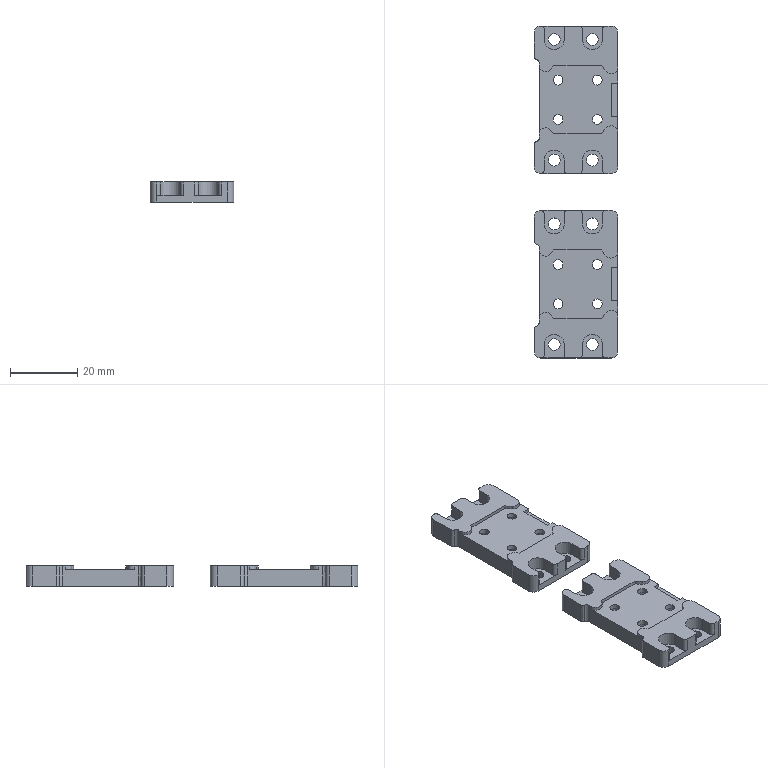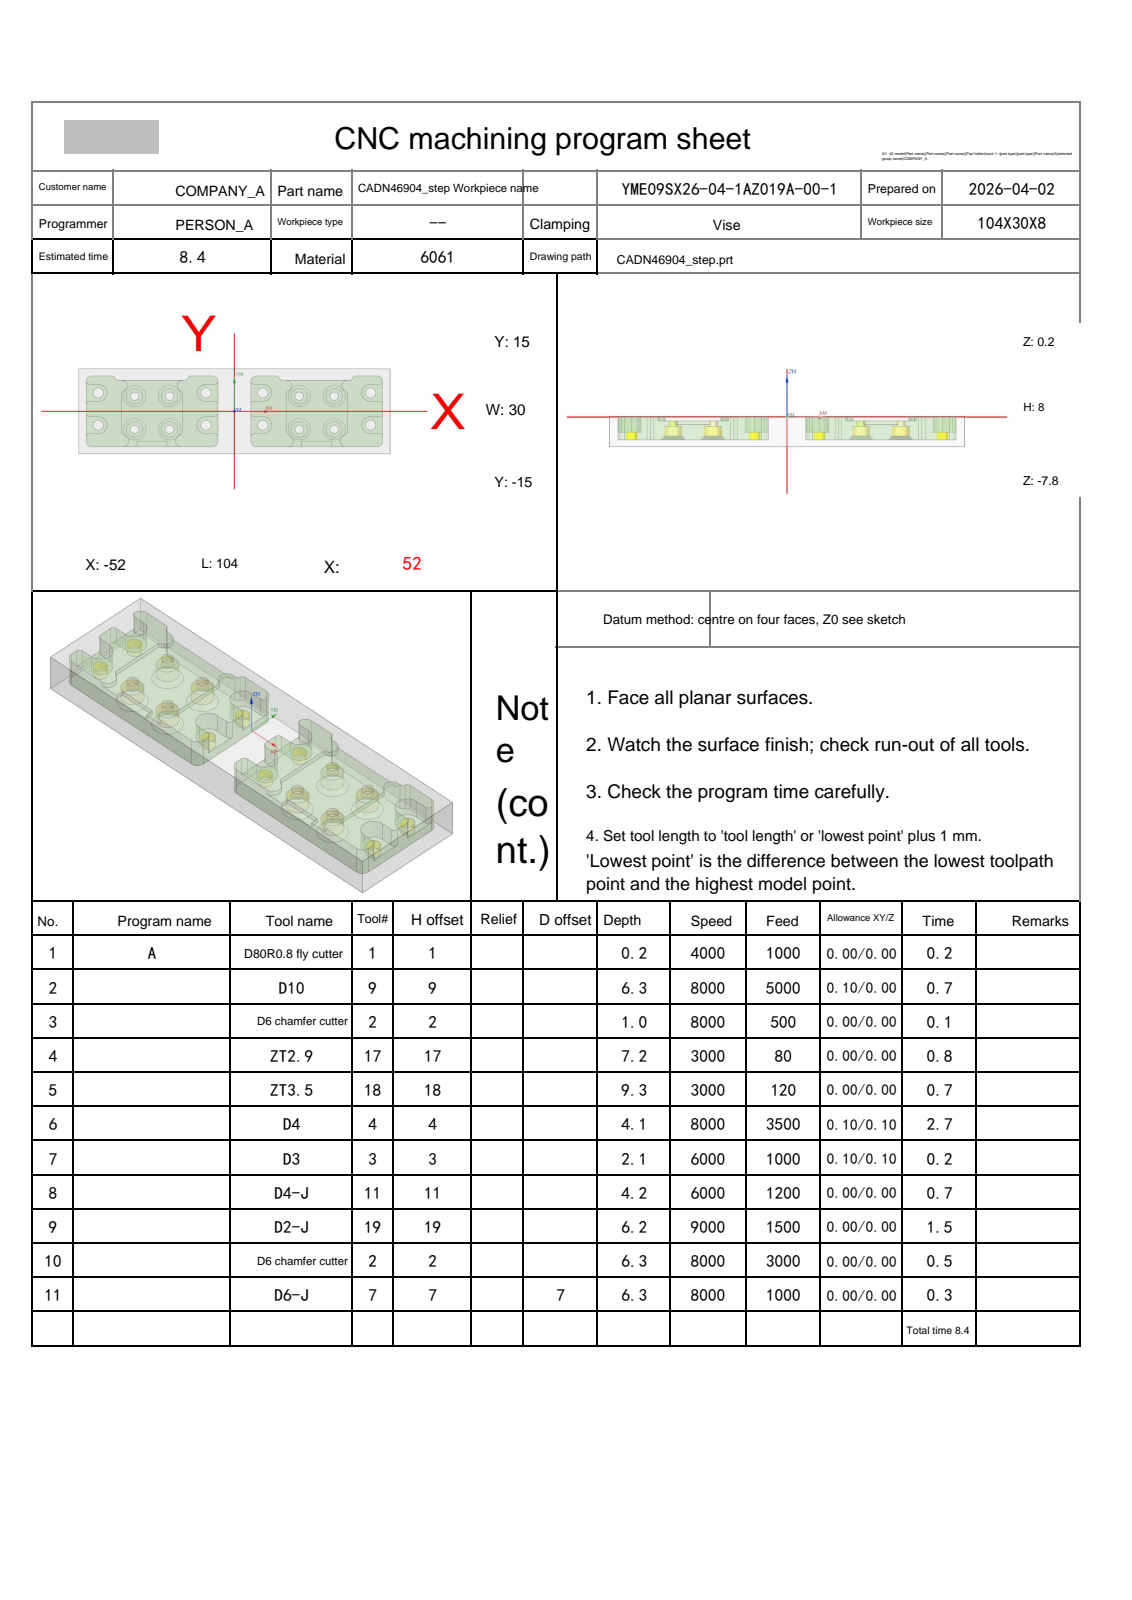NC program | NX | posted by the shop | part box 25 x 99 x 6 mm
Lines 8968 to 9316 of 9316:
N10 T02 M06
(D6 chamfer cutter  D=6. R=0. H=02 ce=0.00 di=0.00)
G00 G90 G54 X36.322 Y-.75 M03 S8000
G43 H02 Z20.
M08
Z2.849
G01 Z-.7 F3000.
G03 X36.622 Y-.83 I.3 J.52
X37.142 Y-.53 I0.0 J.6
G01 X37.15 Y-.5
Y6.325
X36.667 Y6.677
X36.201 Y7.053
G02 X35.297 Y9. I1.646 J1.947
X36.976 Y11.397 I2.55 J0.0
G01 X37.405 Y11.511
X37.847 Y11.55
X38.5
X38.646 Y11.574
X38.776 Y11.644
X38.876 Y11.753
X38.936 Y11.887
G02 X40.436 Y13.05 I1.501 J-.387
G01 X47.5
G02 X50.05 Y10.5 I0.0 J-2.55
X48.5 Y8.95 I-1.55 J0.0
G01 X45.5
G03 X43.05 Y6.5 I0.0 J-2.45
X45.5 Y4.05 I2.45 J0.0
G01 X48.5
G02 X50.05 Y2.5 I0.0 J-1.55
G01 Y-.881
G02 X48.5 Y-2.431 I-1.55 J0.0
G01 X45.5
G03 X43.05 Y-4.881 I0.0 J-2.45
X45.5 Y-7.331 I2.45 J0.0
G01 X48.5
G02 X50.05 Y-8.881 I0.0 J-1.55
G01 Y-10.5
G02 X47.5 Y-13.05 I-2.55 J0.0
G01 X37.298
G02 X34.748 Y-10.5 I0.0 J2.55
X35.009 Y-9.375 I2.55 J0.0
G01 X35.231 Y-9.006
X35.512 Y-8.68
X36.032 Y-8.198
X36.579 Y-7.745
X37.15 Y-7.325
Y-.5
X37.142 Y-.47
G03 X36.622 Y-.17 I-.52 J-.3
X36.322 Y-.25 I0.0 J-.6
G01 Z2.849
G00 Z20.
X18.678
Z2.849
G01 Z-.7
G03 X18.378 Y-.17 I-.3 J-.52
X17.858 Y-.47 I0.0 J-.6
G01 X17.85 Y-.5
Y-7.325
X18.421 Y-7.745
X18.968 Y-8.198
X19.488 Y-8.68
G02 X20.252 Y-10.5 I-1.786 J-1.82
X18.547 Y-12.906 I-2.55 J0.0
G01 X18.131 Y-13.014
X17.702 Y-13.05
X7.5
G02 X4.95 Y-10.5 I0.0 J2.55
G01 Y-8.881
G02 X6.5 Y-7.331 I1.55 J0.0
G01 X9.5
G03 X11.95 Y-4.881 I0.0 J2.45
X9.5 Y-2.431 I-2.45 J0.0
G01 X6.5
G02 X4.95 Y-.881 I0.0 J1.55
G01 Y2.5
G02 X6.5 Y4.05 I1.55 J0.0
G01 X9.5
G03 X11.95 Y6.5 I0.0 J2.45
X9.5 Y8.95 I-2.45 J0.0
G01 X6.5
G02 X4.95 Y10.5 I0.0 J1.55
X7.5 Y13.05 I2.55 J0.0
G01 X14.064
G02 X15.564 Y11.888 I0.0 J-1.55
G01 X15.624 Y11.753
X15.724 Y11.644
X15.854 Y11.574
X16. Y11.55
X17.153
G02 X19.703 Y9. I0.0 J-2.55
X19.366 Y7.732 I-2.55 J0.0
G01 X19.112 Y7.367
X18.799 Y7.053
X18.333 Y6.677
X17.85 Y6.325
Y-.5
X17.858 Y-.53
G03 X18.378 Y-.83 I.52 J.3
X18.678 Y-.75 I0.0 J.6
G01 Z2.849
G00 Z20.
X-18.678
Z2.849
G01 Z-.7
G03 X-18.378 Y-.83 I.3 J.52
X-17.858 Y-.53 I0.0 J.6
G01 X-17.85 Y-.5
Y6.325
X-18.333 Y6.677
X-18.799 Y7.053
G02 X-19.703 Y9. I1.646 J1.947
X-18.024 Y11.397 I2.55 J0.0
G01 X-17.595 Y11.511
X-17.153 Y11.55
X-16.5
X-16.354 Y11.574
X-16.224 Y11.644
X-16.124 Y11.753
X-16.064 Y11.887
G02 X-14.564 Y13.05 I1.501 J-.387
G01 X-7.5
G02 X-4.95 Y10.5 I0.0 J-2.55
X-6.5 Y8.95 I-1.55 J0.0
G01 X-9.5
G03 X-11.95 Y6.5 I0.0 J-2.45
X-9.5 Y4.05 I2.45 J0.0
G01 X-6.5
G02 X-4.95 Y2.5 I0.0 J-1.55
G01 Y-.881
G02 X-6.5 Y-2.431 I-1.55 J0.0
G01 X-9.5
G03 X-11.95 Y-4.881 I0.0 J-2.45
X-9.5 Y-7.331 I2.45 J0.0
G01 X-6.5
G02 X-4.95 Y-8.881 I0.0 J-1.55
G01 Y-10.5
G02 X-7.5 Y-13.05 I-2.55 J0.0
G01 X-17.702
G02 X-20.252 Y-10.5 I0.0 J2.55
X-19.991 Y-9.375 I2.55 J0.0
G01 X-19.769 Y-9.006
X-19.488 Y-8.68
X-18.968 Y-8.198
X-18.421 Y-7.745
X-17.85 Y-7.325
Y-.5
X-17.858 Y-.47
G03 X-18.378 Y-.17 I-.52 J-.3
X-18.678 Y-.25 I0.0 J-.6
G01 Z2.849
G00 Z20.
X-36.322
Z2.849
G01 Z-.7
G03 X-36.622 Y-.17 I-.3 J-.52
X-37.142 Y-.47 I0.0 J-.6
G01 X-37.15 Y-.5
Y-7.325
X-36.579 Y-7.745
X-36.032 Y-8.198
X-35.512 Y-8.68
G02 X-34.748 Y-10.5 I-1.786 J-1.82
X-36.453 Y-12.906 I-2.55 J0.0
G01 X-36.869 Y-13.014
X-37.298 Y-13.05
X-47.5
G02 X-50.05 Y-10.5 I0.0 J2.55
G01 Y-8.881
G02 X-48.5 Y-7.331 I1.55 J0.0
G01 X-45.5
G03 X-43.05 Y-4.881 I0.0 J2.45
X-45.5 Y-2.431 I-2.45 J0.0
G01 X-48.5
G02 X-50.05 Y-.881 I0.0 J1.55
G01 Y2.5
G02 X-48.5 Y4.05 I1.55 J0.0
G01 X-45.5
G03 X-43.05 Y6.5 I0.0 J2.45
X-45.5 Y8.95 I-2.45 J0.0
G01 X-48.5
G02 X-50.05 Y10.5 I0.0 J1.55
X-47.5 Y13.05 I2.55 J0.0
G01 X-40.936
G02 X-39.436 Y11.888 I0.0 J-1.55
G01 X-39.376 Y11.753
X-39.276 Y11.644
X-39.146 Y11.574
X-39. Y11.55
X-37.847
G02 X-35.297 Y9. I0.0 J-2.55
X-35.634 Y7.732 I-2.55 J0.0
G01 X-35.888 Y7.367
X-36.201 Y7.053
X-36.667 Y6.677
X-37.15 Y6.325
Y-.5
X-37.142 Y-.53
G03 X-36.622 Y-.83 I.52 J.3
X-36.322 Y-.75 I0.0 J.6
G01 Z2.849
G00 Z20.
X-20.363 Y-13.05
Z2.541
G01 Z-1.7
X-22.5
G02 X-23.05 Y-12.5 I0.0 J.55
G01 Y-11.05
X-31.95
Y-12.5
G02 X-32.5 Y-13.05 I-.55 J0.0
G01 X-34.637
Z2.541
G00 Z20.
X-35.254 Y11.798
Z2.505
G01 Z-1.7
X-35.278 Y11.708
X-35.188 Y11.552
X-35.179 Y11.55
X-19.821
X-19.812 Y11.552
X-19.722 Y11.708
X-19.746 Y11.798
Z2.505
G00 Z20.
X34.637 Y-13.05
Z2.541
G01 Z-1.7
X32.5
G02 X31.95 Y-12.5 I0.0 J.55
G01 Y-11.05
X23.05
Y-12.5
G02 X22.5 Y-13.05 I-.55 J0.0
G01 X20.363
Z2.541
G00 Z20.
X19.746 Y11.798
Z2.505
G01 Z-1.7
X19.722 Y11.708
X19.812 Y11.552
X19.821 Y11.55
X35.179
X35.188 Y11.552
X35.278 Y11.708
X35.254 Y11.798
Z2.505
G00 Z20.
X30.898 Y-13.05
Z1.534
G01 Z-2.7
X24.102
Z1.534
G00 Z20.
X-24.102
Z1.534
G01 Z-2.7
X-30.898
Z1.534
G00 Z20.
G00 G90 X-33.338 Y5.329 M03 S8000
Z20.
G98 G81 X-33.338 Y5.329 Z-2.75 R2. F500.
X-33.329 Y-6.338
X-21.662 Y-6.33
X-21.671 Y5.329
X21.662
X33.329
X33.338 Y-6.33
X21.671 Y-6.338
G80
G00 Z20.
G00 G90 X-45.5 Y-4.881 M03 S8000
Z20.
G98 G81 X-45.5 Y-4.881 Z-6.05 R-1. F500.
Y6.5
X-9.5
Y-4.881
X9.5
Y6.5
X45.5
Y-4.881
G80
G00 Z20.
G91 G28 Z0.0
M05
M09
G91 G28 Z0.0
M01
N11 T07 M06
(D6-J  D=6. R=0. H=07 ce=0.00 di=0.00)
G00 G90 G54 X-6.487 Y-16.616 M03 S8000
G43 H07 Z20.
M08
Z-5.6
G01 Z-6.1 F1000.
G41 D07
X-6.503 Y-16.417
G03 X-7.5 Y-15.5 I-.997 J-.083
G01 X-47.5
G02 X-52.5 Y-10.5 I0.0 J5.
G01 Y10.5
G02 X-47.5 Y15.5 I5. J0.0
G01 X-40.936
G02 X-37.814 Y14. I0.0 J-4.
G01 X-17.686
G02 X-14.564 Y15.5 I3.122 J-2.5
G01 X-7.5
G02 X-2.5 Y10.5 I0.0 J-5.
G01 Y-10.5
G02 X-7.5 Y-15.5 I-5. J0.0
G01 X-8.
G03 X-9. Y-16.5 I0.0 J-1.
G01 G40 Y-16.7
Z-5.6
G00 Z20.
X48.513 Y-16.616
Z-5.6
G01 Z-6.1
G41 D07
X48.497 Y-16.417
G03 X47.5 Y-15.5 I-.997 J-.083
G01 X7.5
G02 X2.5 Y-10.5 I0.0 J5.
G01 Y10.5
G02 X7.5 Y15.5 I5. J0.0
G01 X14.064
G02 X17.186 Y14. I0.0 J-4.
G01 X37.314
G02 X40.436 Y15.5 I3.122 J-2.5
G01 X47.5
G02 X52.5 Y10.5 I0.0 J-5.
G01 Y-10.5
G02 X47.5 Y-15.5 I-5. J0.0
G01 X47.
G03 X46. Y-16.5 I0.0 J-1.
G01 G40 Y-16.7
Z-5.6
G00 Z20.
M05
M09
G91 G28 Z0.0
G91 G28 Y0.0
M30
%